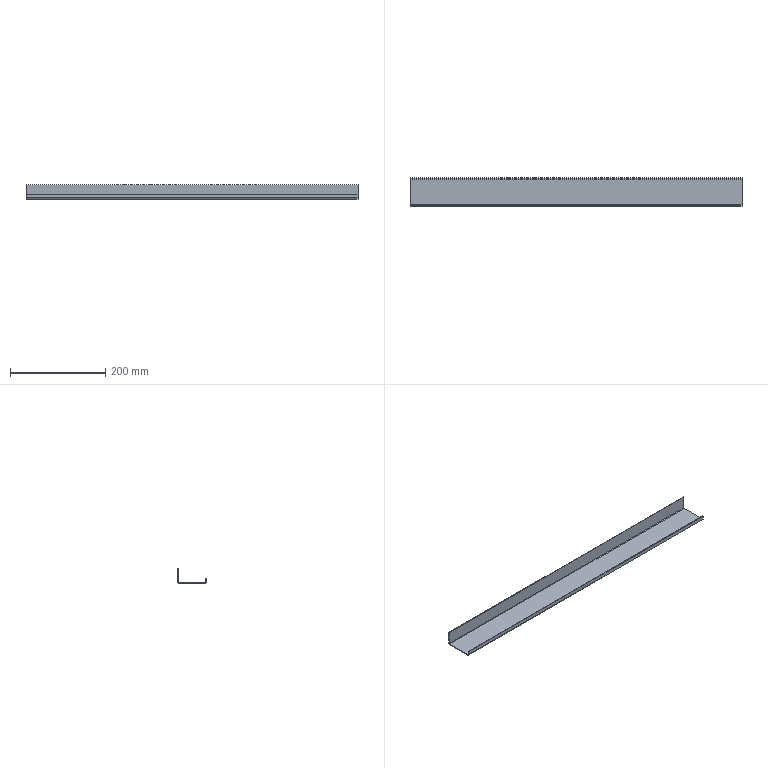Part | STEP file | 1 solid | 22 faces | box 697 x 59 x 30 mm | volume 98797 mm3 | plane 18 | cylinder 4 | commonest cylinder face diameters 2 x2 5 x2
STEP:
#1=CARTESIAN_POINT('',(0.,0.,0.));
#2=DIRECTION('',(0.,0.,1.));
#3=DIRECTION('',(1.,0.,0.));
#4=AXIS2_PLACEMENT_3D('',#1,#2,#3);
#5=CARTESIAN_POINT('',(697.,-56.5,-28.5));
#6=VERTEX_POINT('',#5);
#7=CARTESIAN_POINT('',(697.,-56.5,-30.));
#8=VERTEX_POINT('',#7);
#9=CARTESIAN_POINT('',(697.,-56.5,-28.5));
#10=DIRECTION('',(0.,0.,-1.));
#11=VECTOR('',#10,1.);
#12=LINE('',#9,#11);
#13=CARTESIAN_POINT('',(697.,-59.,-30.));
#14=DIRECTION('',(-1.,0.,0.));
#15=DIRECTION('',(0.,0.,1.));
#16=AXIS2_PLACEMENT_3D('',#13,#14,#15);
#17=PLANE('',#16);
#18=CARTESIAN_POINT('',(1.5,2.5));
#19=DIRECTION('',(-1.,0.));
#20=VECTOR('',#19,1.);
#21=LINE('',#18,#20);
#22=(GEOMETRIC_REPRESENTATION_CONTEXT(2)PARAMETRIC_REPRESENTATION_CONTEXT()REPRESENTATION_CONTEXT('',''));
#23=DEFINITIONAL_REPRESENTATION('',(#21),#22);
#24=PCURVE('',#17,#23);
#25=CARTESIAN_POINT('',(697.,-56.5,-27.5));
#26=DIRECTION('',(-1.,0.,0.));
#27=DIRECTION('',(0.,0.,1.));
#28=AXIS2_PLACEMENT_3D('',#25,#26,#27);
#29=PLANE('',#28);
#30=CARTESIAN_POINT('',(-1.,0.));
#31=DIRECTION('',(-1.,0.));
#32=VECTOR('',#31,1.);
#33=LINE('',#30,#32);
#34=(GEOMETRIC_REPRESENTATION_CONTEXT(2)PARAMETRIC_REPRESENTATION_CONTEXT()REPRESENTATION_CONTEXT('',''));
#35=DEFINITIONAL_REPRESENTATION('',(#33),#34);
#36=PCURVE('',#29,#35);
#37=SURFACE_CURVE('',#12,(#24,#36),.PCURVE_S1.);
#38=EDGE_CURVE('',#6,#8,#37,.T.);
#39=ORIENTED_EDGE('',*,*,#38,.T.);
#40=CARTESIAN_POINT('',(697.,-2.5,-30.));
#41=VERTEX_POINT('',#40);
#42=CARTESIAN_POINT('',(697.,0.,-30.));
#43=DIRECTION('',(0.,-1.,0.));
#44=VECTOR('',#43,1.);
#45=LINE('',#42,#44);
#46=CARTESIAN_POINT('',(0.,59.));
#47=DIRECTION('',(0.,-1.));
#48=VECTOR('',#47,1.);
#49=LINE('',#46,#48);
#50=(GEOMETRIC_REPRESENTATION_CONTEXT(2)PARAMETRIC_REPRESENTATION_CONTEXT()REPRESENTATION_CONTEXT('',''));
#51=DEFINITIONAL_REPRESENTATION('',(#49),#50);
#52=PCURVE('',#17,#51);
#53=CARTESIAN_POINT('',(0.,0.,-30.));
#54=DIRECTION('',(0.,0.,1.));
#55=DIRECTION('',(0.,-1.,0.));
#56=AXIS2_PLACEMENT_3D('',#53,#54,#55);
#57=PLANE('',#56);
#58=CARTESIAN_POINT('',(0.,697.));
#59=DIRECTION('',(1.,0.));
#60=VECTOR('',#59,1.);
#61=LINE('',#58,#60);
#62=(GEOMETRIC_REPRESENTATION_CONTEXT(2)PARAMETRIC_REPRESENTATION_CONTEXT()REPRESENTATION_CONTEXT('',''));
#63=DEFINITIONAL_REPRESENTATION('',(#61),#62);
#64=PCURVE('',#57,#63);
#65=SURFACE_CURVE('',#45,(#52,#64),.PCURVE_S1.);
#66=EDGE_CURVE('',#41,#8,#65,.T.);
#67=ORIENTED_EDGE('',*,*,#66,.F.);
#68=CARTESIAN_POINT('',(697.,-2.5,-28.5));
#69=VERTEX_POINT('',#68);
#70=CARTESIAN_POINT('',(697.,-2.5,-28.5));
#71=DIRECTION('',(0.,0.,-1.));
#72=VECTOR('',#71,1.);
#73=LINE('',#70,#72);
#74=CARTESIAN_POINT('',(1.5,56.5));
#75=DIRECTION('',(-1.,0.));
#76=VECTOR('',#75,1.);
#77=LINE('',#74,#76);
#78=(GEOMETRIC_REPRESENTATION_CONTEXT(2)PARAMETRIC_REPRESENTATION_CONTEXT()REPRESENTATION_CONTEXT('',''));
#79=DEFINITIONAL_REPRESENTATION('',(#77),#78);
#80=PCURVE('',#17,#79);
#81=CARTESIAN_POINT('',(697.,-2.5,-27.5));
#82=DIRECTION('',(-1.,0.,0.));
#83=DIRECTION('',(0.,0.,1.));
#84=AXIS2_PLACEMENT_3D('',#81,#82,#83);
#85=PLANE('',#84);
#86=CARTESIAN_POINT('',(-1.,0.));
#87=DIRECTION('',(-1.,0.));
#88=VECTOR('',#87,1.);
#89=LINE('',#86,#88);
#90=(GEOMETRIC_REPRESENTATION_CONTEXT(2)PARAMETRIC_REPRESENTATION_CONTEXT()REPRESENTATION_CONTEXT('',''));
#91=DEFINITIONAL_REPRESENTATION('',(#89),#90);
#92=PCURVE('',#85,#91);
#93=SURFACE_CURVE('',#73,(#80,#92),.PCURVE_S1.);
#94=EDGE_CURVE('',#69,#41,#93,.T.);
#95=ORIENTED_EDGE('',*,*,#94,.F.);
#96=CARTESIAN_POINT('',(697.,-59.,-28.5));
#97=DIRECTION('',(0.,-1.,0.));
#98=VECTOR('',#97,1.);
#99=LINE('',#96,#98);
#100=CARTESIAN_POINT('',(1.5,0.));
#101=DIRECTION('',(0.,-1.));
#102=VECTOR('',#101,1.);
#103=LINE('',#100,#102);
#104=(GEOMETRIC_REPRESENTATION_CONTEXT(2)PARAMETRIC_REPRESENTATION_CONTEXT()REPRESENTATION_CONTEXT('',''));
#105=DEFINITIONAL_REPRESENTATION('',(#103),#104);
#106=PCURVE('',#17,#105);
#107=CARTESIAN_POINT('',(0.,0.,-28.5));
#108=DIRECTION('',(0.,0.,1.));
#109=DIRECTION('',(0.,-1.,0.));
#110=AXIS2_PLACEMENT_3D('',#107,#108,#109);
#111=PLANE('',#110);
#112=CARTESIAN_POINT('',(59.,697.));
#113=DIRECTION('',(1.,0.));
#114=VECTOR('',#113,1.);
#115=LINE('',#112,#114);
#116=(GEOMETRIC_REPRESENTATION_CONTEXT(2)PARAMETRIC_REPRESENTATION_CONTEXT()REPRESENTATION_CONTEXT('',''));
#117=DEFINITIONAL_REPRESENTATION('',(#115),#116);
#118=PCURVE('',#111,#117);
#119=SURFACE_CURVE('',#99,(#106,#118),.PCURVE_S1.);
#120=EDGE_CURVE('',#69,#6,#119,.T.);
#121=ORIENTED_EDGE('',*,*,#120,.T.);
#122=EDGE_LOOP('',(#39,#67,#95,#121));
#123=FACE_BOUND('',#122,.T.);
#124=ADVANCED_FACE('',(#123),#17,.F.);
#125=CARTESIAN_POINT('',(0.,-56.5,-28.5));
#126=VERTEX_POINT('',#125);
#127=CARTESIAN_POINT('',(0.,-56.5,-30.));
#128=VERTEX_POINT('',#127);
#129=CARTESIAN_POINT('',(0.,-56.5,-28.5));
#130=DIRECTION('',(0.,0.,-1.));
#131=VECTOR('',#130,1.);
#132=LINE('',#129,#131);
#133=CARTESIAN_POINT('',(0.,-1.5,-30.));
#134=DIRECTION('',(1.,0.,0.));
#135=DIRECTION('',(0.,1.,0.));
#136=AXIS2_PLACEMENT_3D('',#133,#134,#135);
#137=PLANE('',#136);
#138=CARTESIAN_POINT('',(-55.,1.5));
#139=DIRECTION('',(0.,-1.));
#140=VECTOR('',#139,1.);
#141=LINE('',#138,#140);
#142=(GEOMETRIC_REPRESENTATION_CONTEXT(2)PARAMETRIC_REPRESENTATION_CONTEXT()REPRESENTATION_CONTEXT('',''));
#143=DEFINITIONAL_REPRESENTATION('',(#141),#142);
#144=PCURVE('',#137,#143);
#145=CARTESIAN_POINT('',(0.,-56.5,-27.5));
#146=DIRECTION('',(-1.,0.,0.));
#147=DIRECTION('',(0.,0.,1.));
#148=AXIS2_PLACEMENT_3D('',#145,#146,#147);
#149=PLANE('',#148);
#150=CARTESIAN_POINT('',(-1.,0.));
#151=DIRECTION('',(-1.,0.));
#152=VECTOR('',#151,1.);
#153=LINE('',#150,#152);
#154=(GEOMETRIC_REPRESENTATION_CONTEXT(2)PARAMETRIC_REPRESENTATION_CONTEXT()REPRESENTATION_CONTEXT('',''));
#155=DEFINITIONAL_REPRESENTATION('',(#153),#154);
#156=PCURVE('',#149,#155);
#157=SURFACE_CURVE('',#132,(#144,#156),.PCURVE_S1.);
#158=EDGE_CURVE('',#126,#128,#157,.T.);
#159=ORIENTED_EDGE('',*,*,#158,.F.);
#160=CARTESIAN_POINT('',(0.,-2.5,-28.5));
#161=VERTEX_POINT('',#160);
#162=CARTESIAN_POINT('',(0.,-1.5,-28.5));
#163=DIRECTION('',(0.,1.,0.));
#164=VECTOR('',#163,1.);
#165=LINE('',#162,#164);
#166=CARTESIAN_POINT('',(0.,1.5));
#167=DIRECTION('',(1.,0.));
#168=VECTOR('',#167,1.);
#169=LINE('',#166,#168);
#170=(GEOMETRIC_REPRESENTATION_CONTEXT(2)PARAMETRIC_REPRESENTATION_CONTEXT()REPRESENTATION_CONTEXT('',''));
#171=DEFINITIONAL_REPRESENTATION('',(#169),#170);
#172=PCURVE('',#137,#171);
#173=CARTESIAN_POINT('',(1.5,0.));
#174=DIRECTION('',(-1.,0.));
#175=VECTOR('',#174,1.);
#176=LINE('',#173,#175);
#177=(GEOMETRIC_REPRESENTATION_CONTEXT(2)PARAMETRIC_REPRESENTATION_CONTEXT()REPRESENTATION_CONTEXT('',''));
#178=DEFINITIONAL_REPRESENTATION('',(#176),#177);
#179=PCURVE('',#111,#178);
#180=SURFACE_CURVE('',#165,(#172,#179),.PCURVE_S1.);
#181=EDGE_CURVE('',#126,#161,#180,.T.);
#182=ORIENTED_EDGE('',*,*,#181,.T.);
#183=CARTESIAN_POINT('',(0.,-2.5,-30.));
#184=VERTEX_POINT('',#183);
#185=CARTESIAN_POINT('',(0.,-2.5,-30.));
#186=DIRECTION('',(0.,0.,-1.));
#187=VECTOR('',#186,1.);
#188=LINE('',#185,#187);
#189=CARTESIAN_POINT('',(-1.,0.));
#190=DIRECTION('',(0.,-1.));
#191=VECTOR('',#190,1.);
#192=LINE('',#189,#191);
#193=(GEOMETRIC_REPRESENTATION_CONTEXT(2)PARAMETRIC_REPRESENTATION_CONTEXT()REPRESENTATION_CONTEXT('',''));
#194=DEFINITIONAL_REPRESENTATION('',(#192),#193);
#195=PCURVE('',#137,#194);
#196=CARTESIAN_POINT('',(0.,-2.5,-27.5));
#197=DIRECTION('',(-1.,0.,0.));
#198=DIRECTION('',(0.,0.,1.));
#199=AXIS2_PLACEMENT_3D('',#196,#197,#198);
#200=PLANE('',#199);
#201=CARTESIAN_POINT('',(-2.5,0.));
#202=DIRECTION('',(-1.,0.));
#203=VECTOR('',#202,1.);
#204=LINE('',#201,#203);
#205=(GEOMETRIC_REPRESENTATION_CONTEXT(2)PARAMETRIC_REPRESENTATION_CONTEXT()REPRESENTATION_CONTEXT('',''));
#206=DEFINITIONAL_REPRESENTATION('',(#204),#205);
#207=PCURVE('',#200,#206);
#208=SURFACE_CURVE('',#188,(#195,#207),.PCURVE_S1.);
#209=EDGE_CURVE('',#161,#184,#208,.T.);
#210=ORIENTED_EDGE('',*,*,#209,.T.);
#211=CARTESIAN_POINT('',(0.,0.,-30.));
#212=DIRECTION('',(0.,1.,0.));
#213=VECTOR('',#212,1.);
#214=LINE('',#211,#213);
#215=CARTESIAN_POINT('',(1.5,0.));
#216=DIRECTION('',(1.,0.));
#217=VECTOR('',#216,1.);
#218=LINE('',#215,#217);
#219=(GEOMETRIC_REPRESENTATION_CONTEXT(2)PARAMETRIC_REPRESENTATION_CONTEXT()REPRESENTATION_CONTEXT('',''));
#220=DEFINITIONAL_REPRESENTATION('',(#218),#219);
#221=PCURVE('',#137,#220);
#222=CARTESIAN_POINT('',(0.,0.));
#223=DIRECTION('',(-1.,0.));
#224=VECTOR('',#223,1.);
#225=LINE('',#222,#224);
#226=(GEOMETRIC_REPRESENTATION_CONTEXT(2)PARAMETRIC_REPRESENTATION_CONTEXT()REPRESENTATION_CONTEXT('',''));
#227=DEFINITIONAL_REPRESENTATION('',(#225),#226);
#228=PCURVE('',#57,#227);
#229=SURFACE_CURVE('',#214,(#221,#228),.PCURVE_S1.);
#230=EDGE_CURVE('',#128,#184,#229,.T.);
#231=ORIENTED_EDGE('',*,*,#230,.F.);
#232=EDGE_LOOP('',(#159,#182,#210,#231));
#233=FACE_BOUND('',#232,.T.);
#234=ADVANCED_FACE('',(#233),#137,.F.);
#235=CARTESIAN_POINT('',(697.,-56.5,-30.));
#236=DIRECTION('',(-1.,0.,0.));
#237=VECTOR('',#236,1.);
#238=LINE('',#235,#237);
#239=CARTESIAN_POINT('',(56.5,697.));
#240=DIRECTION('',(0.,-1.));
#241=VECTOR('',#240,1.);
#242=LINE('',#239,#241);
#243=(GEOMETRIC_REPRESENTATION_CONTEXT(2)PARAMETRIC_REPRESENTATION_CONTEXT()REPRESENTATION_CONTEXT('',''));
#244=DEFINITIONAL_REPRESENTATION('',(#242),#243);
#245=PCURVE('',#57,#244);
#246=CARTESIAN_POINT('',(697.,-56.5,-27.5));
#247=DIRECTION('',(1.,0.,0.));
#248=DIRECTION('',(0.,-1.,0.));
#249=AXIS2_PLACEMENT_3D('',#246,#247,#248);
#250=CYLINDRICAL_SURFACE('',#249,2.5);
#251=CARTESIAN_POINT('',(1.571,0.));
#252=DIRECTION('',(0.,-1.));
#253=VECTOR('',#252,1.);
#254=LINE('',#251,#253);
#255=(GEOMETRIC_REPRESENTATION_CONTEXT(2)PARAMETRIC_REPRESENTATION_CONTEXT()REPRESENTATION_CONTEXT('',''));
#256=DEFINITIONAL_REPRESENTATION('',(#254),#255);
#257=PCURVE('',#250,#256);
#258=SURFACE_CURVE('',#238,(#245,#257),.PCURVE_S1.);
#259=EDGE_CURVE('',#8,#128,#258,.T.);
#260=ORIENTED_EDGE('',*,*,#259,.T.);
#261=ORIENTED_EDGE('',*,*,#230,.T.);
#262=CARTESIAN_POINT('',(0.,-2.5,-30.));
#263=DIRECTION('',(-1.,0.,0.));
#264=VECTOR('',#263,1.);
#265=LINE('',#262,#264);
#266=CARTESIAN_POINT('',(2.5,0.));
#267=DIRECTION('',(0.,-1.));
#268=VECTOR('',#267,1.);
#269=LINE('',#266,#268);
#270=(GEOMETRIC_REPRESENTATION_CONTEXT(2)PARAMETRIC_REPRESENTATION_CONTEXT()REPRESENTATION_CONTEXT('',''));
#271=DEFINITIONAL_REPRESENTATION('',(#269),#270);
#272=PCURVE('',#57,#271);
#273=CARTESIAN_POINT('',(697.,-2.5,-27.5));
#274=DIRECTION('',(1.,0.,0.));
#275=DIRECTION('',(0.,0.,-1.));
#276=AXIS2_PLACEMENT_3D('',#273,#274,#275);
#277=CYLINDRICAL_SURFACE('',#276,2.5);
#278=CARTESIAN_POINT('',(0.,-697.));
#279=DIRECTION('',(0.,-1.));
#280=VECTOR('',#279,1.);
#281=LINE('',#278,#280);
#282=(GEOMETRIC_REPRESENTATION_CONTEXT(2)PARAMETRIC_REPRESENTATION_CONTEXT()REPRESENTATION_CONTEXT('',''));
#283=DEFINITIONAL_REPRESENTATION('',(#281),#282);
#284=PCURVE('',#277,#283);
#285=SURFACE_CURVE('',#265,(#272,#284),.PCURVE_S1.);
#286=EDGE_CURVE('',#41,#184,#285,.T.);
#287=ORIENTED_EDGE('',*,*,#286,.F.);
#288=ORIENTED_EDGE('',*,*,#66,.T.);
#289=EDGE_LOOP('',(#260,#261,#287,#288));
#290=FACE_BOUND('',#289,.T.);
#291=ADVANCED_FACE('',(#290),#57,.F.);
#292=ORIENTED_EDGE('',*,*,#181,.F.);
#293=CARTESIAN_POINT('',(697.,-56.5,-28.5));
#294=DIRECTION('',(-1.,0.,0.));
#295=VECTOR('',#294,1.);
#296=LINE('',#293,#295);
#297=CARTESIAN_POINT('',(56.5,697.));
#298=DIRECTION('',(0.,-1.));
#299=VECTOR('',#298,1.);
#300=LINE('',#297,#299);
#301=(GEOMETRIC_REPRESENTATION_CONTEXT(2)PARAMETRIC_REPRESENTATION_CONTEXT()REPRESENTATION_CONTEXT('',''));
#302=DEFINITIONAL_REPRESENTATION('',(#300),#301);
#303=PCURVE('',#111,#302);
#304=CARTESIAN_POINT('',(697.,-56.5,-27.5));
#305=DIRECTION('',(1.,0.,0.));
#306=DIRECTION('',(0.,-1.,0.));
#307=AXIS2_PLACEMENT_3D('',#304,#305,#306);
#308=CYLINDRICAL_SURFACE('',#307,1.);
#309=CARTESIAN_POINT('',(1.571,0.));
#310=DIRECTION('',(0.,-1.));
#311=VECTOR('',#310,1.);
#312=LINE('',#309,#311);
#313=(GEOMETRIC_REPRESENTATION_CONTEXT(2)PARAMETRIC_REPRESENTATION_CONTEXT()REPRESENTATION_CONTEXT('',''));
#314=DEFINITIONAL_REPRESENTATION('',(#312),#313);
#315=PCURVE('',#308,#314);
#316=SURFACE_CURVE('',#296,(#303,#315),.PCURVE_S1.);
#317=EDGE_CURVE('',#6,#126,#316,.T.);
#318=ORIENTED_EDGE('',*,*,#317,.F.);
#319=ORIENTED_EDGE('',*,*,#120,.F.);
#320=CARTESIAN_POINT('',(0.,-2.5,-28.5));
#321=DIRECTION('',(1.,0.,0.));
#322=VECTOR('',#321,1.);
#323=LINE('',#320,#322);
#324=CARTESIAN_POINT('',(2.5,0.));
#325=DIRECTION('',(0.,1.));
#326=VECTOR('',#325,1.);
#327=LINE('',#324,#326);
#328=(GEOMETRIC_REPRESENTATION_CONTEXT(2)PARAMETRIC_REPRESENTATION_CONTEXT()REPRESENTATION_CONTEXT('',''));
#329=DEFINITIONAL_REPRESENTATION('',(#327),#328);
#330=PCURVE('',#111,#329);
#331=CARTESIAN_POINT('',(697.,-2.5,-27.5));
#332=DIRECTION('',(1.,0.,0.));
#333=DIRECTION('',(0.,0.,-1.));
#334=AXIS2_PLACEMENT_3D('',#331,#332,#333);
#335=CYLINDRICAL_SURFACE('',#334,1.);
#336=CARTESIAN_POINT('',(0.,-697.));
#337=DIRECTION('',(0.,1.));
#338=VECTOR('',#337,1.);
#339=LINE('',#336,#338);
#340=(GEOMETRIC_REPRESENTATION_CONTEXT(2)PARAMETRIC_REPRESENTATION_CONTEXT()REPRESENTATION_CONTEXT('',''));
#341=DEFINITIONAL_REPRESENTATION('',(#339),#340);
#342=PCURVE('',#335,#341);
#343=SURFACE_CURVE('',#323,(#330,#342),.PCURVE_S1.);
#344=EDGE_CURVE('',#161,#69,#343,.T.);
#345=ORIENTED_EDGE('',*,*,#344,.F.);
#346=EDGE_LOOP('',(#292,#318,#319,#345));
#347=FACE_BOUND('',#346,.T.);
#348=ADVANCED_FACE('',(#347),#111,.T.);
#349=CARTESIAN_POINT('',(697.,-1.5,0.));
#350=VERTEX_POINT('',#349);
#351=CARTESIAN_POINT('',(697.,-1.5,-27.5));
#352=VERTEX_POINT('',#351);
#353=CARTESIAN_POINT('',(697.,-1.5,-30.));
#354=DIRECTION('',(0.,0.,-1.));
#355=VECTOR('',#354,1.);
#356=LINE('',#353,#355);
#357=CARTESIAN_POINT('',(697.,-1.5,-30.));
#358=DIRECTION('',(1.,0.,0.));
#359=DIRECTION('',(0.,0.,-1.));
#360=AXIS2_PLACEMENT_3D('',#357,#358,#359);
#361=PLANE('',#360);
#362=CARTESIAN_POINT('',(0.,0.));
#363=DIRECTION('',(1.,0.));
#364=VECTOR('',#363,1.);
#365=LINE('',#362,#364);
#366=(GEOMETRIC_REPRESENTATION_CONTEXT(2)PARAMETRIC_REPRESENTATION_CONTEXT()REPRESENTATION_CONTEXT('',''));
#367=DEFINITIONAL_REPRESENTATION('',(#365),#366);
#368=PCURVE('',#361,#367);
#369=CARTESIAN_POINT('',(0.,-1.5,0.));
#370=DIRECTION('',(0.,1.,0.));
#371=DIRECTION('',(0.,0.,1.));
#372=AXIS2_PLACEMENT_3D('',#369,#370,#371);
#373=PLANE('',#372);
#374=CARTESIAN_POINT('',(-30.,697.));
#375=DIRECTION('',(-1.,0.));
#376=VECTOR('',#375,1.);
#377=LINE('',#374,#376);
#378=(GEOMETRIC_REPRESENTATION_CONTEXT(2)PARAMETRIC_REPRESENTATION_CONTEXT()REPRESENTATION_CONTEXT('',''));
#379=DEFINITIONAL_REPRESENTATION('',(#377),#378);
#380=PCURVE('',#373,#379);
#381=SURFACE_CURVE('',#356,(#368,#380),.PCURVE_S1.);
#382=EDGE_CURVE('',#350,#352,#381,.T.);
#383=ORIENTED_EDGE('',*,*,#382,.T.);
#384=CARTESIAN_POINT('',(697.,0.,-27.5));
#385=VERTEX_POINT('',#384);
#386=CARTESIAN_POINT('',(697.,-1.5,-27.5));
#387=DIRECTION('',(0.,1.,0.));
#388=VECTOR('',#387,1.);
#389=LINE('',#386,#388);
#390=CARTESIAN_POINT('',(-2.5,0.));
#391=DIRECTION('',(0.,1.));
#392=VECTOR('',#391,1.);
#393=LINE('',#390,#392);
#394=(GEOMETRIC_REPRESENTATION_CONTEXT(2)PARAMETRIC_REPRESENTATION_CONTEXT()REPRESENTATION_CONTEXT('',''));
#395=DEFINITIONAL_REPRESENTATION('',(#393),#394);
#396=PCURVE('',#361,#395);
#397=CARTESIAN_POINT('',(0.,1.));
#398=DIRECTION('',(0.,1.));
#399=VECTOR('',#398,1.);
#400=LINE('',#397,#399);
#401=(GEOMETRIC_REPRESENTATION_CONTEXT(2)PARAMETRIC_REPRESENTATION_CONTEXT()REPRESENTATION_CONTEXT('',''));
#402=DEFINITIONAL_REPRESENTATION('',(#400),#401);
#403=PCURVE('',#85,#402);
#404=SURFACE_CURVE('',#389,(#396,#403),.PCURVE_S1.);
#405=EDGE_CURVE('',#352,#385,#404,.T.);
#406=ORIENTED_EDGE('',*,*,#405,.T.);
#407=CARTESIAN_POINT('',(697.,0.,0.));
#408=VERTEX_POINT('',#407);
#409=CARTESIAN_POINT('',(697.,0.,-30.));
#410=DIRECTION('',(0.,0.,-1.));
#411=VECTOR('',#410,1.);
#412=LINE('',#409,#411);
#413=CARTESIAN_POINT('',(0.,1.5));
#414=DIRECTION('',(1.,0.));
#415=VECTOR('',#414,1.);
#416=LINE('',#413,#415);
#417=(GEOMETRIC_REPRESENTATION_CONTEXT(2)PARAMETRIC_REPRESENTATION_CONTEXT()REPRESENTATION_CONTEXT('',''));
#418=DEFINITIONAL_REPRESENTATION('',(#416),#417);
#419=PCURVE('',#361,#418);
#420=CARTESIAN_POINT('',(0.,0.,0.));
#421=DIRECTION('',(0.,1.,0.));
#422=DIRECTION('',(0.,0.,1.));
#423=AXIS2_PLACEMENT_3D('',#420,#421,#422);
#424=PLANE('',#423);
#425=CARTESIAN_POINT('',(-30.,697.));
#426=DIRECTION('',(-1.,0.));
#427=VECTOR('',#426,1.);
#428=LINE('',#425,#427);
#429=(GEOMETRIC_REPRESENTATION_CONTEXT(2)PARAMETRIC_REPRESENTATION_CONTEXT()REPRESENTATION_CONTEXT('',''));
#430=DEFINITIONAL_REPRESENTATION('',(#428),#429);
#431=PCURVE('',#424,#430);
#432=SURFACE_CURVE('',#412,(#419,#431),.PCURVE_S1.);
#433=EDGE_CURVE('',#408,#385,#432,.T.);
#434=ORIENTED_EDGE('',*,*,#433,.F.);
#435=CARTESIAN_POINT('',(697.,-1.5,0.));
#436=DIRECTION('',(0.,1.,0.));
#437=VECTOR('',#436,1.);
#438=LINE('',#435,#437);
#439=CARTESIAN_POINT('',(-30.,0.));
#440=DIRECTION('',(0.,1.));
#441=VECTOR('',#440,1.);
#442=LINE('',#439,#441);
#443=(GEOMETRIC_REPRESENTATION_CONTEXT(2)PARAMETRIC_REPRESENTATION_CONTEXT()REPRESENTATION_CONTEXT('',''));
#444=DEFINITIONAL_REPRESENTATION('',(#442),#443);
#445=PCURVE('',#361,#444);
#446=CARTESIAN_POINT('',(0.,-1.5,0.));
#447=DIRECTION('',(0.,0.,1.));
#448=DIRECTION('',(1.,0.,0.));
#449=AXIS2_PLACEMENT_3D('',#446,#447,#448);
#450=PLANE('',#449);
#451=CARTESIAN_POINT('',(697.,0.));
#452=DIRECTION('',(0.,1.));
#453=VECTOR('',#452,1.);
#454=LINE('',#451,#453);
#455=(GEOMETRIC_REPRESENTATION_CONTEXT(2)PARAMETRIC_REPRESENTATION_CONTEXT()REPRESENTATION_CONTEXT('',''));
#456=DEFINITIONAL_REPRESENTATION('',(#454),#455);
#457=PCURVE('',#450,#456);
#458=SURFACE_CURVE('',#438,(#445,#457),.PCURVE_S1.);
#459=EDGE_CURVE('',#350,#408,#458,.T.);
#460=ORIENTED_EDGE('',*,*,#459,.F.);
#461=EDGE_LOOP('',(#383,#406,#434,#460));
#462=FACE_BOUND('',#461,.T.);
#463=ADVANCED_FACE('',(#462),#361,.T.);
#464=CARTESIAN_POINT('',(0.,-1.5,-27.5));
#465=VERTEX_POINT('',#464);
#466=CARTESIAN_POINT('',(697.,-1.5,-27.5));
#467=DIRECTION('',(-1.,0.,0.));
#468=VECTOR('',#467,1.);
#469=LINE('',#466,#468);
#470=CARTESIAN_POINT('',(-27.5,697.));
#471=DIRECTION('',(0.,-1.));
#472=VECTOR('',#471,1.);
#473=LINE('',#470,#472);
#474=(GEOMETRIC_REPRESENTATION_CONTEXT(2)PARAMETRIC_REPRESENTATION_CONTEXT()REPRESENTATION_CONTEXT('',''));
#475=DEFINITIONAL_REPRESENTATION('',(#473),#474);
#476=PCURVE('',#373,#475);
#477=CARTESIAN_POINT('',(1.571,0.));
#478=DIRECTION('',(0.,-1.));
#479=VECTOR('',#478,1.);
#480=LINE('',#477,#479);
#481=(GEOMETRIC_REPRESENTATION_CONTEXT(2)PARAMETRIC_REPRESENTATION_CONTEXT()REPRESENTATION_CONTEXT('',''));
#482=DEFINITIONAL_REPRESENTATION('',(#480),#481);
#483=PCURVE('',#335,#482);
#484=SURFACE_CURVE('',#469,(#476,#483),.PCURVE_S1.);
#485=EDGE_CURVE('',#352,#465,#484,.T.);
#486=ORIENTED_EDGE('',*,*,#485,.F.);
#487=ORIENTED_EDGE('',*,*,#382,.F.);
#488=CARTESIAN_POINT('',(0.,-1.5,0.));
#489=VERTEX_POINT('',#488);
#490=CARTESIAN_POINT('',(0.,-1.5,0.));
#491=DIRECTION('',(1.,0.,0.));
#492=VECTOR('',#491,1.);
#493=LINE('',#490,#492);
#494=CARTESIAN_POINT('',(0.,0.));
#495=DIRECTION('',(0.,1.));
#496=VECTOR('',#495,1.);
#497=LINE('',#494,#496);
#498=(GEOMETRIC_REPRESENTATION_CONTEXT(2)PARAMETRIC_REPRESENTATION_CONTEXT()REPRESENTATION_CONTEXT('',''));
#499=DEFINITIONAL_REPRESENTATION('',(#497),#498);
#500=PCURVE('',#373,#499);
#501=CARTESIAN_POINT('',(0.,0.));
#502=DIRECTION('',(1.,0.));
#503=VECTOR('',#502,1.);
#504=LINE('',#501,#503);
#505=(GEOMETRIC_REPRESENTATION_CONTEXT(2)PARAMETRIC_REPRESENTATION_CONTEXT()REPRESENTATION_CONTEXT('',''));
#506=DEFINITIONAL_REPRESENTATION('',(#504),#505);
#507=PCURVE('',#450,#506);
#508=SURFACE_CURVE('',#493,(#500,#507),.PCURVE_S1.);
#509=EDGE_CURVE('',#489,#350,#508,.T.);
#510=ORIENTED_EDGE('',*,*,#509,.F.);
#511=CARTESIAN_POINT('',(0.,-1.5,-30.));
#512=DIRECTION('',(0.,0.,1.));
#513=VECTOR('',#512,1.);
#514=LINE('',#511,#513);
#515=CARTESIAN_POINT('',(-30.,0.));
#516=DIRECTION('',(1.,0.));
#517=VECTOR('',#516,1.);
#518=LINE('',#515,#517);
#519=(GEOMETRIC_REPRESENTATION_CONTEXT(2)PARAMETRIC_REPRESENTATION_CONTEXT()REPRESENTATION_CONTEXT('',''));
#520=DEFINITIONAL_REPRESENTATION('',(#518),#519);
#521=PCURVE('',#373,#520);
#522=CARTESIAN_POINT('',(0.,-1.5,-30.));
#523=DIRECTION('',(-1.,0.,0.));
#524=DIRECTION('',(0.,0.,1.));
#525=AXIS2_PLACEMENT_3D('',#522,#523,#524);
#526=PLANE('',#525);
#527=CARTESIAN_POINT('',(0.,0.));
#528=DIRECTION('',(1.,0.));
#529=VECTOR('',#528,1.);
#530=LINE('',#527,#529);
#531=(GEOMETRIC_REPRESENTATION_CONTEXT(2)PARAMETRIC_REPRESENTATION_CONTEXT()REPRESENTATION_CONTEXT('',''));
#532=DEFINITIONAL_REPRESENTATION('',(#530),#531);
#533=PCURVE('',#526,#532);
#534=SURFACE_CURVE('',#514,(#521,#533),.PCURVE_S1.);
#535=EDGE_CURVE('',#465,#489,#534,.T.);
#536=ORIENTED_EDGE('',*,*,#535,.F.);
#537=EDGE_LOOP('',(#486,#487,#510,#536));
#538=FACE_BOUND('',#537,.T.);
#539=ADVANCED_FACE('',(#538),#373,.F.);
#540=ORIENTED_EDGE('',*,*,#433,.T.);
#541=CARTESIAN_POINT('',(0.,0.,-27.5));
#542=VERTEX_POINT('',#541);
#543=CARTESIAN_POINT('',(697.,0.,-27.5));
#544=DIRECTION('',(-1.,0.,0.));
#545=VECTOR('',#544,1.);
#546=LINE('',#543,#545);
#547=CARTESIAN_POINT('',(-27.5,697.));
#548=DIRECTION('',(0.,-1.));
#549=VECTOR('',#548,1.);
#550=LINE('',#547,#549);
#551=(GEOMETRIC_REPRESENTATION_CONTEXT(2)PARAMETRIC_REPRESENTATION_CONTEXT()REPRESENTATION_CONTEXT('',''));
#552=DEFINITIONAL_REPRESENTATION('',(#550),#551);
#553=PCURVE('',#424,#552);
#554=CARTESIAN_POINT('',(1.571,0.));
#555=DIRECTION('',(0.,-1.));
#556=VECTOR('',#555,1.);
#557=LINE('',#554,#556);
#558=(GEOMETRIC_REPRESENTATION_CONTEXT(2)PARAMETRIC_REPRESENTATION_CONTEXT()REPRESENTATION_CONTEXT('',''));
#559=DEFINITIONAL_REPRESENTATION('',(#557),#558);
#560=PCURVE('',#277,#559);
#561=SURFACE_CURVE('',#546,(#553,#560),.PCURVE_S1.);
#562=EDGE_CURVE('',#385,#542,#561,.T.);
#563=ORIENTED_EDGE('',*,*,#562,.T.);
#564=CARTESIAN_POINT('',(0.,0.,0.));
#565=VERTEX_POINT('',#564);
#566=CARTESIAN_POINT('',(0.,0.,-30.));
#567=DIRECTION('',(0.,0.,1.));
#568=VECTOR('',#567,1.);
#569=LINE('',#566,#568);
#570=CARTESIAN_POINT('',(-30.,0.));
#571=DIRECTION('',(1.,0.));
#572=VECTOR('',#571,1.);
#573=LINE('',#570,#572);
#574=(GEOMETRIC_REPRESENTATION_CONTEXT(2)PARAMETRIC_REPRESENTATION_CONTEXT()REPRESENTATION_CONTEXT('',''));
#575=DEFINITIONAL_REPRESENTATION('',(#573),#574);
#576=PCURVE('',#424,#575);
#577=CARTESIAN_POINT('',(0.,1.5));
#578=DIRECTION('',(1.,0.));
#579=VECTOR('',#578,1.);
#580=LINE('',#577,#579);
#581=(GEOMETRIC_REPRESENTATION_CONTEXT(2)PARAMETRIC_REPRESENTATION_CONTEXT()REPRESENTATION_CONTEXT('',''));
#582=DEFINITIONAL_REPRESENTATION('',(#580),#581);
#583=PCURVE('',#526,#582);
#584=SURFACE_CURVE('',#569,(#576,#583),.PCURVE_S1.);
#585=EDGE_CURVE('',#542,#565,#584,.T.);
#586=ORIENTED_EDGE('',*,*,#585,.T.);
#587=CARTESIAN_POINT('',(0.,0.,0.));
#588=DIRECTION('',(1.,0.,0.));
#589=VECTOR('',#588,1.);
#590=LINE('',#587,#589);
#591=CARTESIAN_POINT('',(0.,0.));
#592=DIRECTION('',(0.,1.));
#593=VECTOR('',#592,1.);
#594=LINE('',#591,#593);
#595=(GEOMETRIC_REPRESENTATION_CONTEXT(2)PARAMETRIC_REPRESENTATION_CONTEXT()REPRESENTATION_CONTEXT('',''));
#596=DEFINITIONAL_REPRESENTATION('',(#594),#595);
#597=PCURVE('',#424,#596);
#598=CARTESIAN_POINT('',(0.,1.5));
#599=DIRECTION('',(1.,0.));
#600=VECTOR('',#599,1.);
#601=LINE('',#598,#600);
#602=(GEOMETRIC_REPRESENTATION_CONTEXT(2)PARAMETRIC_REPRESENTATION_CONTEXT()REPRESENTATION_CONTEXT('',''));
#603=DEFINITIONAL_REPRESENTATION('',(#601),#602);
#604=PCURVE('',#450,#603);
#605=SURFACE_CURVE('',#590,(#597,#604),.PCURVE_S1.);
#606=EDGE_CURVE('',#565,#408,#605,.T.);
#607=ORIENTED_EDGE('',*,*,#606,.T.);
#608=EDGE_LOOP('',(#540,#563,#586,#607));
#609=FACE_BOUND('',#608,.T.);
#610=ADVANCED_FACE('',(#609),#424,.T.);
#611=CARTESIAN_POINT('',(0.,-1.5,-27.5));
#612=DIRECTION('',(0.,1.,0.));
#613=VECTOR('',#612,1.);
#614=LINE('',#611,#613);
#615=CARTESIAN_POINT('',(2.5,0.));
#616=DIRECTION('',(0.,1.));
#617=VECTOR('',#616,1.);
#618=LINE('',#615,#617);
#619=(GEOMETRIC_REPRESENTATION_CONTEXT(2)PARAMETRIC_REPRESENTATION_CONTEXT()REPRESENTATION_CONTEXT('',''));
#620=DEFINITIONAL_REPRESENTATION('',(#618),#619);
#621=PCURVE('',#526,#620);
#622=CARTESIAN_POINT('',(0.,1.));
#623=DIRECTION('',(0.,1.));
#624=VECTOR('',#623,1.);
#625=LINE('',#622,#624);
#626=(GEOMETRIC_REPRESENTATION_CONTEXT(2)PARAMETRIC_REPRESENTATION_CONTEXT()REPRESENTATION_CONTEXT('',''));
#627=DEFINITIONAL_REPRESENTATION('',(#625),#626);
#628=PCURVE('',#200,#627);
#629=SURFACE_CURVE('',#614,(#621,#628),.PCURVE_S1.);
#630=EDGE_CURVE('',#465,#542,#629,.T.);
#631=ORIENTED_EDGE('',*,*,#630,.F.);
#632=ORIENTED_EDGE('',*,*,#535,.T.);
#633=CARTESIAN_POINT('',(0.,-1.5,0.));
#634=DIRECTION('',(0.,1.,0.));
#635=VECTOR('',#634,1.);
#636=LINE('',#633,#635);
#637=CARTESIAN_POINT('',(30.,0.));
#638=DIRECTION('',(0.,1.));
#639=VECTOR('',#638,1.);
#640=LINE('',#637,#639);
#641=(GEOMETRIC_REPRESENTATION_CONTEXT(2)PARAMETRIC_REPRESENTATION_CONTEXT()REPRESENTATION_CONTEXT('',''));
#642=DEFINITIONAL_REPRESENTATION('',(#640),#641);
#643=PCURVE('',#526,#642);
#644=CARTESIAN_POINT('',(0.,0.));
#645=DIRECTION('',(0.,1.));
#646=VECTOR('',#645,1.);
#647=LINE('',#644,#646);
#648=(GEOMETRIC_REPRESENTATION_CONTEXT(2)PARAMETRIC_REPRESENTATION_CONTEXT()REPRESENTATION_CONTEXT('',''));
#649=DEFINITIONAL_REPRESENTATION('',(#647),#648);
#650=PCURVE('',#450,#649);
#651=SURFACE_CURVE('',#636,(#643,#650),.PCURVE_S1.);
#652=EDGE_CURVE('',#489,#565,#651,.T.);
#653=ORIENTED_EDGE('',*,*,#652,.T.);
#654=ORIENTED_EDGE('',*,*,#585,.F.);
#655=EDGE_LOOP('',(#631,#632,#653,#654));
#656=FACE_BOUND('',#655,.T.);
#657=ADVANCED_FACE('',(#656),#526,.T.);
#658=ORIENTED_EDGE('',*,*,#606,.F.);
#659=ORIENTED_EDGE('',*,*,#652,.F.);
#660=ORIENTED_EDGE('',*,*,#509,.T.);
#661=ORIENTED_EDGE('',*,*,#459,.T.);
#662=EDGE_LOOP('',(#658,#659,#660,#661));
#663=FACE_BOUND('',#662,.T.);
#664=ADVANCED_FACE('',(#663),#450,.T.);
#665=ORIENTED_EDGE('',*,*,#209,.F.);
#666=CARTESIAN_POINT('',(0.,-2.5,-27.5));
#667=DIRECTION('',(-1.,0.,0.));
#668=DIRECTION('',(0.,0.,-1.));
#669=AXIS2_PLACEMENT_3D('',#666,#667,#668);
#670=CIRCLE('',#669,1.);
#671=CARTESIAN_POINT('',(0.,0.));
#672=DIRECTION('',(-1.,0.));
#673=AXIS2_PLACEMENT_2D('',#671,#672);
#674=CIRCLE('',#673,1.);
#675=(GEOMETRIC_REPRESENTATION_CONTEXT(2)PARAMETRIC_REPRESENTATION_CONTEXT()REPRESENTATION_CONTEXT('',''));
#676=DEFINITIONAL_REPRESENTATION('',(#674),#675);
#677=PCURVE('',#200,#676);
#678=CARTESIAN_POINT('',(6.283,-697.));
#679=DIRECTION('',(-1.,0.));
#680=VECTOR('',#679,1.);
#681=LINE('',#678,#680);
#682=(GEOMETRIC_REPRESENTATION_CONTEXT(2)PARAMETRIC_REPRESENTATION_CONTEXT()REPRESENTATION_CONTEXT('',''));
#683=DEFINITIONAL_REPRESENTATION('',(#681),#682);
#684=PCURVE('',#335,#683);
#685=SURFACE_CURVE('',#670,(#677,#684),.PCURVE_S1.);
#686=EDGE_CURVE('',#465,#161,#685,.T.);
#687=ORIENTED_EDGE('',*,*,#686,.F.);
#688=ORIENTED_EDGE('',*,*,#630,.T.);
#689=CARTESIAN_POINT('',(0.,-2.5,-27.5));
#690=DIRECTION('',(-1.,0.,0.));
#691=DIRECTION('',(0.,0.,-1.));
#692=AXIS2_PLACEMENT_3D('',#689,#690,#691);
#693=CIRCLE('',#692,2.5);
#694=CARTESIAN_POINT('',(0.,0.));
#695=DIRECTION('',(-1.,0.));
#696=AXIS2_PLACEMENT_2D('',#694,#695);
#697=CIRCLE('',#696,2.5);
#698=(GEOMETRIC_REPRESENTATION_CONTEXT(2)PARAMETRIC_REPRESENTATION_CONTEXT()REPRESENTATION_CONTEXT('',''));
#699=DEFINITIONAL_REPRESENTATION('',(#697),#698);
#700=PCURVE('',#200,#699);
#701=CARTESIAN_POINT('',(6.283,-697.));
#702=DIRECTION('',(-1.,0.));
#703=VECTOR('',#702,1.);
#704=LINE('',#701,#703);
#705=(GEOMETRIC_REPRESENTATION_CONTEXT(2)PARAMETRIC_REPRESENTATION_CONTEXT()REPRESENTATION_CONTEXT('',''));
#706=DEFINITIONAL_REPRESENTATION('',(#704),#705);
#707=PCURVE('',#277,#706);
#708=SURFACE_CURVE('',#693,(#700,#707),.PCURVE_S1.);
#709=EDGE_CURVE('',#542,#184,#708,.T.);
#710=ORIENTED_EDGE('',*,*,#709,.T.);
#711=EDGE_LOOP('',(#665,#687,#688,#710));
#712=FACE_BOUND('',#711,.T.);
#713=ADVANCED_FACE('',(#712),#200,.T.);
#714=CARTESIAN_POINT('',(697.,-2.5,-27.5));
#715=DIRECTION('',(1.,0.,0.));
#716=DIRECTION('',(0.,0.,-1.));
#717=AXIS2_PLACEMENT_3D('',#714,#715,#716);
#718=CIRCLE('',#717,1.);
#719=CARTESIAN_POINT('',(-1.,0.));
#720=CARTESIAN_POINT('',(-1.,1.732));
#721=CARTESIAN_POINT('',(0.5,0.866));
#722=CARTESIAN_POINT('',(2.,0.));
#723=CARTESIAN_POINT('',(0.5,-0.866));
#724=CARTESIAN_POINT('',(-1.,-1.732));
#725=CARTESIAN_POINT('',(-1.,0.));
#726=(BOUNDED_CURVE()B_SPLINE_CURVE(2,(#719,#720,#721,#722,#723,#724,#725),.UNSPECIFIED.,.T.,.F.)B_SPLINE_CURVE_WITH_KNOTS((1,2,2,2,2,1),(-2.094,0.,2.094,4.189,6.283,8.378),.UNSPECIFIED.)CURVE()GEOMETRIC_REPRESENTATION_ITEM()RATIONAL_B_SPLINE_CURVE((1.,0.5,1.,0.5,1.,0.5,1.))REPRESENTATION_ITEM(''));
#727=(GEOMETRIC_REPRESENTATION_CONTEXT(2)PARAMETRIC_REPRESENTATION_CONTEXT()REPRESENTATION_CONTEXT('',''));
#728=DEFINITIONAL_REPRESENTATION('',(#726),#727);
#729=PCURVE('',#85,#728);
#730=CARTESIAN_POINT('',(0.,0.));
#731=DIRECTION('',(1.,0.));
#732=VECTOR('',#731,1.);
#733=LINE('',#730,#732);
#734=(GEOMETRIC_REPRESENTATION_CONTEXT(2)PARAMETRIC_REPRESENTATION_CONTEXT()REPRESENTATION_CONTEXT('',''));
#735=DEFINITIONAL_REPRESENTATION('',(#733),#734);
#736=PCURVE('',#335,#735);
#737=SURFACE_CURVE('',#718,(#729,#736),.PCURVE_S1.);
#738=EDGE_CURVE('',#69,#352,#737,.T.);
#739=ORIENTED_EDGE('',*,*,#738,.F.);
#740=ORIENTED_EDGE('',*,*,#94,.T.);
#741=CARTESIAN_POINT('',(697.,-2.5,-27.5));
#742=DIRECTION('',(1.,0.,0.));
#743=DIRECTION('',(0.,0.,-1.));
#744=AXIS2_PLACEMENT_3D('',#741,#742,#743);
#745=CIRCLE('',#744,2.5);
#746=CARTESIAN_POINT('',(-2.5,0.));
#747=CARTESIAN_POINT('',(-2.5,4.33));
#748=CARTESIAN_POINT('',(1.25,2.165));
#749=CARTESIAN_POINT('',(5.,0.));
#750=CARTESIAN_POINT('',(1.25,-2.165));
#751=CARTESIAN_POINT('',(-2.5,-4.33));
#752=CARTESIAN_POINT('',(-2.5,0.));
#753=(BOUNDED_CURVE()B_SPLINE_CURVE(2,(#746,#747,#748,#749,#750,#751,#752),.UNSPECIFIED.,.T.,.F.)B_SPLINE_CURVE_WITH_KNOTS((1,2,2,2,2,1),(-2.094,0.,2.094,4.189,6.283,8.378),.UNSPECIFIED.)CURVE()GEOMETRIC_REPRESENTATION_ITEM()RATIONAL_B_SPLINE_CURVE((1.,0.5,1.,0.5,1.,0.5,1.))REPRESENTATION_ITEM(''));
#754=(GEOMETRIC_REPRESENTATION_CONTEXT(2)PARAMETRIC_REPRESENTATION_CONTEXT()REPRESENTATION_CONTEXT('',''));
#755=DEFINITIONAL_REPRESENTATION('',(#753),#754);
#756=PCURVE('',#85,#755);
#757=CARTESIAN_POINT('',(0.,0.));
#758=DIRECTION('',(1.,0.));
#759=VECTOR('',#758,1.);
#760=LINE('',#757,#759);
#761=(GEOMETRIC_REPRESENTATION_CONTEXT(2)PARAMETRIC_REPRESENTATION_CONTEXT()REPRESENTATION_CONTEXT('',''));
#762=DEFINITIONAL_REPRESENTATION('',(#760),#761);
#763=PCURVE('',#277,#762);
#764=SURFACE_CURVE('',#745,(#756,#763),.PCURVE_S1.);
#765=EDGE_CURVE('',#41,#385,#764,.T.);
#766=ORIENTED_EDGE('',*,*,#765,.T.);
#767=ORIENTED_EDGE('',*,*,#405,.F.);
#768=EDGE_LOOP('',(#739,#740,#766,#767));
#769=FACE_BOUND('',#768,.T.);
#770=ADVANCED_FACE('',(#769),#85,.F.);
#771=ORIENTED_EDGE('',*,*,#562,.F.);
#772=ORIENTED_EDGE('',*,*,#765,.F.);
#773=ORIENTED_EDGE('',*,*,#286,.T.);
#774=ORIENTED_EDGE('',*,*,#709,.F.);
#775=EDGE_LOOP('',(#771,#772,#773,#774));
#776=FACE_BOUND('',#775,.T.);
#777=ADVANCED_FACE('',(#776),#277,.T.);
#778=ORIENTED_EDGE('',*,*,#738,.F.);
#779=ORIENTED_EDGE('',*,*,#344,.F.);
#780=ORIENTED_EDGE('',*,*,#686,.F.);
#781=ORIENTED_EDGE('',*,*,#485,.F.);
#782=EDGE_LOOP('',(#778,#779,#780,#781));
#783=FACE_BOUND('',#782,.F.);
#784=ADVANCED_FACE('',(#783),#335,.F.);
#785=CARTESIAN_POINT('',(0.,-57.5,-27.5));
#786=VERTEX_POINT('',#785);
#787=CARTESIAN_POINT('',(0.,-59.,-27.5));
#788=VERTEX_POINT('',#787);
#789=CARTESIAN_POINT('',(0.,-59.,-27.5));
#790=DIRECTION('',(0.,-1.,0.));
#791=VECTOR('',#790,1.);
#792=LINE('',#789,#791);
#793=CARTESIAN_POINT('',(0.,-2.5));
#794=DIRECTION('',(0.,-1.));
#795=VECTOR('',#794,1.);
#796=LINE('',#793,#795);
#797=(GEOMETRIC_REPRESENTATION_CONTEXT(2)PARAMETRIC_REPRESENTATION_CONTEXT()REPRESENTATION_CONTEXT('',''));
#798=DEFINITIONAL_REPRESENTATION('',(#796),#797);
#799=PCURVE('',#149,#798);
#800=CARTESIAN_POINT('',(0.,-59.,-28.5));
#801=DIRECTION('',(1.,0.,0.));
#802=DIRECTION('',(0.,0.,-1.));
#803=AXIS2_PLACEMENT_3D('',#800,#801,#802);
#804=PLANE('',#803);
#805=CARTESIAN_POINT('',(-1.,0.));
#806=DIRECTION('',(0.,-1.));
#807=VECTOR('',#806,1.);
#808=LINE('',#805,#807);
#809=(GEOMETRIC_REPRESENTATION_CONTEXT(2)PARAMETRIC_REPRESENTATION_CONTEXT()REPRESENTATION_CONTEXT('',''));
#810=DEFINITIONAL_REPRESENTATION('',(#808),#809);
#811=PCURVE('',#804,#810);
#812=SURFACE_CURVE('',#792,(#799,#811),.PCURVE_S1.);
#813=EDGE_CURVE('',#786,#788,#812,.T.);
#814=ORIENTED_EDGE('',*,*,#813,.F.);
#815=CARTESIAN_POINT('',(0.,-56.5,-27.5));
#816=DIRECTION('',(-1.,0.,0.));
#817=DIRECTION('',(0.,0.,-1.));
#818=AXIS2_PLACEMENT_3D('',#815,#816,#817);
#819=CIRCLE('',#818,1.);
#820=CARTESIAN_POINT('',(0.,0.));
#821=DIRECTION('',(-1.,0.));
#822=AXIS2_PLACEMENT_2D('',#820,#821);
#823=CIRCLE('',#822,1.);
#824=(GEOMETRIC_REPRESENTATION_CONTEXT(2)PARAMETRIC_REPRESENTATION_CONTEXT()REPRESENTATION_CONTEXT('',''));
#825=DEFINITIONAL_REPRESENTATION('',(#823),#824);
#826=PCURVE('',#149,#825);
#827=CARTESIAN_POINT('',(1.571,-697.));
#828=DIRECTION('',(-1.,0.));
#829=VECTOR('',#828,1.);
#830=LINE('',#827,#829);
#831=(GEOMETRIC_REPRESENTATION_CONTEXT(2)PARAMETRIC_REPRESENTATION_CONTEXT()REPRESENTATION_CONTEXT('',''));
#832=DEFINITIONAL_REPRESENTATION('',(#830),#831);
#833=PCURVE('',#308,#832);
#834=SURFACE_CURVE('',#819,(#826,#833),.PCURVE_S1.);
#835=EDGE_CURVE('',#126,#786,#834,.T.);
#836=ORIENTED_EDGE('',*,*,#835,.F.);
#837=ORIENTED_EDGE('',*,*,#158,.T.);
#838=CARTESIAN_POINT('',(0.,-56.5,-27.5));
#839=DIRECTION('',(-1.,0.,0.));
#840=DIRECTION('',(0.,0.,-1.));
#841=AXIS2_PLACEMENT_3D('',#838,#839,#840);
#842=CIRCLE('',#841,2.5);
#843=CARTESIAN_POINT('',(0.,0.));
#844=DIRECTION('',(-1.,0.));
#845=AXIS2_PLACEMENT_2D('',#843,#844);
#846=CIRCLE('',#845,2.5);
#847=(GEOMETRIC_REPRESENTATION_CONTEXT(2)PARAMETRIC_REPRESENTATION_CONTEXT()REPRESENTATION_CONTEXT('',''));
#848=DEFINITIONAL_REPRESENTATION('',(#846),#847);
#849=PCURVE('',#149,#848);
#850=CARTESIAN_POINT('',(1.571,-697.));
#851=DIRECTION('',(-1.,0.));
#852=VECTOR('',#851,1.);
#853=LINE('',#850,#852);
#854=(GEOMETRIC_REPRESENTATION_CONTEXT(2)PARAMETRIC_REPRESENTATION_CONTEXT()REPRESENTATION_CONTEXT('',''));
#855=DEFINITIONAL_REPRESENTATION('',(#853),#854);
#856=PCURVE('',#250,#855);
#857=SURFACE_CURVE('',#842,(#849,#856),.PCURVE_S1.);
#858=EDGE_CURVE('',#128,#788,#857,.T.);
#859=ORIENTED_EDGE('',*,*,#858,.T.);
#860=EDGE_LOOP('',(#814,#836,#837,#859));
#861=FACE_BOUND('',#860,.T.);
#862=ADVANCED_FACE('',(#861),#149,.T.);
#863=CARTESIAN_POINT('',(697.,-57.5,-27.5));
#864=VERTEX_POINT('',#863);
#865=CARTESIAN_POINT('',(697.,-56.5,-27.5));
#866=DIRECTION('',(1.,0.,0.));
#867=DIRECTION('',(0.,0.,-1.));
#868=AXIS2_PLACEMENT_3D('',#865,#866,#867);
#869=CIRCLE('',#868,1.);
#870=CARTESIAN_POINT('',(-1.,0.));
#871=CARTESIAN_POINT('',(-1.,1.732));
#872=CARTESIAN_POINT('',(0.5,0.866));
#873=CARTESIAN_POINT('',(2.,0.));
#874=CARTESIAN_POINT('',(0.5,-0.866));
#875=CARTESIAN_POINT('',(-1.,-1.732));
#876=CARTESIAN_POINT('',(-1.,0.));
#877=(BOUNDED_CURVE()B_SPLINE_CURVE(2,(#870,#871,#872,#873,#874,#875,#876),.UNSPECIFIED.,.T.,.F.)B_SPLINE_CURVE_WITH_KNOTS((1,2,2,2,2,1),(-2.094,0.,2.094,4.189,6.283,8.378),.UNSPECIFIED.)CURVE()GEOMETRIC_REPRESENTATION_ITEM()RATIONAL_B_SPLINE_CURVE((1.,0.5,1.,0.5,1.,0.5,1.))REPRESENTATION_ITEM(''));
#878=(GEOMETRIC_REPRESENTATION_CONTEXT(2)PARAMETRIC_REPRESENTATION_CONTEXT()REPRESENTATION_CONTEXT('',''));
#879=DEFINITIONAL_REPRESENTATION('',(#877),#878);
#880=PCURVE('',#29,#879);
#881=CARTESIAN_POINT('',(-4.712,0.));
#882=DIRECTION('',(1.,0.));
#883=VECTOR('',#882,1.);
#884=LINE('',#881,#883);
#885=(GEOMETRIC_REPRESENTATION_CONTEXT(2)PARAMETRIC_REPRESENTATION_CONTEXT()REPRESENTATION_CONTEXT('',''));
#886=DEFINITIONAL_REPRESENTATION('',(#884),#885);
#887=PCURVE('',#308,#886);
#888=SURFACE_CURVE('',#869,(#880,#887),.PCURVE_S1.);
#889=EDGE_CURVE('',#864,#6,#888,.T.);
#890=ORIENTED_EDGE('',*,*,#889,.F.);
#891=CARTESIAN_POINT('',(697.,-59.,-27.5));
#892=VERTEX_POINT('',#891);
#893=CARTESIAN_POINT('',(697.,-57.5,-27.5));
#894=DIRECTION('',(0.,-1.,0.));
#895=VECTOR('',#894,1.);
#896=LINE('',#893,#895);
#897=CARTESIAN_POINT('',(0.,-1.));
#898=DIRECTION('',(0.,-1.));
#899=VECTOR('',#898,1.);
#900=LINE('',#897,#899);
#901=(GEOMETRIC_REPRESENTATION_CONTEXT(2)PARAMETRIC_REPRESENTATION_CONTEXT()REPRESENTATION_CONTEXT('',''));
#902=DEFINITIONAL_REPRESENTATION('',(#900),#901);
#903=PCURVE('',#29,#902);
#904=CARTESIAN_POINT('',(697.,-59.,-20.));
#905=DIRECTION('',(-1.,0.,0.));
#906=DIRECTION('',(0.,0.,1.));
#907=AXIS2_PLACEMENT_3D('',#904,#905,#906);
#908=PLANE('',#907);
#909=CARTESIAN_POINT('',(-7.5,1.5));
#910=DIRECTION('',(0.,-1.));
#911=VECTOR('',#910,1.);
#912=LINE('',#909,#911);
#913=(GEOMETRIC_REPRESENTATION_CONTEXT(2)PARAMETRIC_REPRESENTATION_CONTEXT()REPRESENTATION_CONTEXT('',''));
#914=DEFINITIONAL_REPRESENTATION('',(#912),#913);
#915=PCURVE('',#908,#914);
#916=SURFACE_CURVE('',#896,(#903,#915),.PCURVE_S1.);
#917=EDGE_CURVE('',#864,#892,#916,.T.);
#918=ORIENTED_EDGE('',*,*,#917,.T.);
#919=CARTESIAN_POINT('',(697.,-56.5,-27.5));
#920=DIRECTION('',(1.,0.,0.));
#921=DIRECTION('',(0.,0.,-1.));
#922=AXIS2_PLACEMENT_3D('',#919,#920,#921);
#923=CIRCLE('',#922,2.5);
#924=CARTESIAN_POINT('',(-2.5,0.));
#925=CARTESIAN_POINT('',(-2.5,4.33));
#926=CARTESIAN_POINT('',(1.25,2.165));
#927=CARTESIAN_POINT('',(5.,0.));
#928=CARTESIAN_POINT('',(1.25,-2.165));
#929=CARTESIAN_POINT('',(-2.5,-4.33));
#930=CARTESIAN_POINT('',(-2.5,0.));
#931=(BOUNDED_CURVE()B_SPLINE_CURVE(2,(#924,#925,#926,#927,#928,#929,#930),.UNSPECIFIED.,.T.,.F.)B_SPLINE_CURVE_WITH_KNOTS((1,2,2,2,2,1),(-2.094,0.,2.094,4.189,6.283,8.378),.UNSPECIFIED.)CURVE()GEOMETRIC_REPRESENTATION_ITEM()RATIONAL_B_SPLINE_CURVE((1.,0.5,1.,0.5,1.,0.5,1.))REPRESENTATION_ITEM(''));
#932=(GEOMETRIC_REPRESENTATION_CONTEXT(2)PARAMETRIC_REPRESENTATION_CONTEXT()REPRESENTATION_CONTEXT('',''));
#933=DEFINITIONAL_REPRESENTATION('',(#931),#932);
#934=PCURVE('',#29,#933);
#935=CARTESIAN_POINT('',(-4.712,0.));
#936=DIRECTION('',(1.,0.));
#937=VECTOR('',#936,1.);
#938=LINE('',#935,#937);
#939=(GEOMETRIC_REPRESENTATION_CONTEXT(2)PARAMETRIC_REPRESENTATION_CONTEXT()REPRESENTATION_CONTEXT('',''));
#940=DEFINITIONAL_REPRESENTATION('',(#938),#939);
#941=PCURVE('',#250,#940);
#942=SURFACE_CURVE('',#923,(#934,#941),.PCURVE_S1.);
#943=EDGE_CURVE('',#892,#8,#942,.T.);
#944=ORIENTED_EDGE('',*,*,#943,.T.);
#945=ORIENTED_EDGE('',*,*,#38,.F.);
#946=EDGE_LOOP('',(#890,#918,#944,#945));
#947=FACE_BOUND('',#946,.T.);
#948=ADVANCED_FACE('',(#947),#29,.F.);
#949=ORIENTED_EDGE('',*,*,#259,.F.);
#950=ORIENTED_EDGE('',*,*,#943,.F.);
#951=CARTESIAN_POINT('',(0.,-59.,-27.5));
#952=DIRECTION('',(-1.,0.,0.));
#953=VECTOR('',#952,1.);
#954=LINE('',#951,#953);
#955=CARTESIAN_POINT('',(0.,-697.));
#956=DIRECTION('',(0.,-1.));
#957=VECTOR('',#956,1.);
#958=LINE('',#955,#957);
#959=(GEOMETRIC_REPRESENTATION_CONTEXT(2)PARAMETRIC_REPRESENTATION_CONTEXT()REPRESENTATION_CONTEXT('',''));
#960=DEFINITIONAL_REPRESENTATION('',(#958),#959);
#961=PCURVE('',#250,#960);
#962=CARTESIAN_POINT('',(0.,-59.,0.));
#963=DIRECTION('',(0.,1.,0.));
#964=DIRECTION('',(0.,0.,1.));
#965=AXIS2_PLACEMENT_3D('',#962,#963,#964);
#966=PLANE('',#965);
#967=CARTESIAN_POINT('',(-27.5,0.));
#968=DIRECTION('',(0.,-1.));
#969=VECTOR('',#968,1.);
#970=LINE('',#967,#969);
#971=(GEOMETRIC_REPRESENTATION_CONTEXT(2)PARAMETRIC_REPRESENTATION_CONTEXT()REPRESENTATION_CONTEXT('',''));
#972=DEFINITIONAL_REPRESENTATION('',(#970),#971);
#973=PCURVE('',#966,#972);
#974=SURFACE_CURVE('',#954,(#961,#973),.PCURVE_S1.);
#975=EDGE_CURVE('',#892,#788,#974,.T.);
#976=ORIENTED_EDGE('',*,*,#975,.T.);
#977=ORIENTED_EDGE('',*,*,#858,.F.);
#978=EDGE_LOOP('',(#949,#950,#976,#977));
#979=FACE_BOUND('',#978,.T.);
#980=ADVANCED_FACE('',(#979),#250,.T.);
#981=ORIENTED_EDGE('',*,*,#889,.F.);
#982=CARTESIAN_POINT('',(0.,-57.5,-27.5));
#983=DIRECTION('',(1.,0.,0.));
#984=VECTOR('',#983,1.);
#985=LINE('',#982,#984);
#986=CARTESIAN_POINT('',(0.,-697.));
#987=DIRECTION('',(0.,1.));
#988=VECTOR('',#987,1.);
#989=LINE('',#986,#988);
#990=(GEOMETRIC_REPRESENTATION_CONTEXT(2)PARAMETRIC_REPRESENTATION_CONTEXT()REPRESENTATION_CONTEXT('',''));
#991=DEFINITIONAL_REPRESENTATION('',(#989),#990);
#992=PCURVE('',#308,#991);
#993=CARTESIAN_POINT('',(0.,-57.5,0.));
#994=DIRECTION('',(0.,1.,0.));
#995=DIRECTION('',(0.,0.,1.));
#996=AXIS2_PLACEMENT_3D('',#993,#994,#995);
#997=PLANE('',#996);
#998=CARTESIAN_POINT('',(-27.5,0.));
#999=DIRECTION('',(0.,1.));
#1000=VECTOR('',#999,1.);
#1001=LINE('',#998,#1000);
#1002=(GEOMETRIC_REPRESENTATION_CONTEXT(2)PARAMETRIC_REPRESENTATION_CONTEXT()REPRESENTATION_CONTEXT('',''));
#1003=DEFINITIONAL_REPRESENTATION('',(#1001),#1002);
#1004=PCURVE('',#997,#1003);
#1005=SURFACE_CURVE('',#985,(#992,#1004),.PCURVE_S1.);
#1006=EDGE_CURVE('',#786,#864,#1005,.T.);
#1007=ORIENTED_EDGE('',*,*,#1006,.F.);
#1008=ORIENTED_EDGE('',*,*,#835,.F.);
#1009=ORIENTED_EDGE('',*,*,#317,.F.);
#1010=EDGE_LOOP('',(#981,#1007,#1008,#1009));
#1011=FACE_BOUND('',#1010,.F.);
#1012=ADVANCED_FACE('',(#1011),#308,.F.);
#1013=ORIENTED_EDGE('',*,*,#917,.F.);
#1014=CARTESIAN_POINT('',(697.,-57.5,-20.));
#1015=VERTEX_POINT('',#1014);
#1016=CARTESIAN_POINT('',(697.,-57.5,-20.));
#1017=DIRECTION('',(0.,0.,1.));
#1018=VECTOR('',#1017,1.);
#1019=LINE('',#1016,#1018);
#1020=CARTESIAN_POINT('',(0.,1.5));
#1021=DIRECTION('',(1.,0.));
#1022=VECTOR('',#1021,1.);
#1023=LINE('',#1020,#1022);
#1024=(GEOMETRIC_REPRESENTATION_CONTEXT(2)PARAMETRIC_REPRESENTATION_CONTEXT()REPRESENTATION_CONTEXT('',''));
#1025=DEFINITIONAL_REPRESENTATION('',(#1023),#1024);
#1026=PCURVE('',#908,#1025);
#1027=CARTESIAN_POINT('',(-20.,697.));
#1028=DIRECTION('',(1.,0.));
#1029=VECTOR('',#1028,1.);
#1030=LINE('',#1027,#1029);
#1031=(GEOMETRIC_REPRESENTATION_CONTEXT(2)PARAMETRIC_REPRESENTATION_CONTEXT()REPRESENTATION_CONTEXT('',''));
#1032=DEFINITIONAL_REPRESENTATION('',(#1030),#1031);
#1033=PCURVE('',#997,#1032);
#1034=SURFACE_CURVE('',#1019,(#1026,#1033),.PCURVE_S1.);
#1035=EDGE_CURVE('',#864,#1015,#1034,.T.);
#1036=ORIENTED_EDGE('',*,*,#1035,.T.);
#1037=CARTESIAN_POINT('',(697.,-59.,-20.));
#1038=VERTEX_POINT('',#1037);
#1039=CARTESIAN_POINT('',(697.,-59.,-20.));
#1040=DIRECTION('',(0.,1.,0.));
#1041=VECTOR('',#1040,1.);
#1042=LINE('',#1039,#1041);
#1043=CARTESIAN_POINT('',(0.,0.));
#1044=DIRECTION('',(0.,1.));
#1045=VECTOR('',#1044,1.);
#1046=LINE('',#1043,#1045);
#1047=(GEOMETRIC_REPRESENTATION_CONTEXT(2)PARAMETRIC_REPRESENTATION_CONTEXT()REPRESENTATION_CONTEXT('',''));
#1048=DEFINITIONAL_REPRESENTATION('',(#1046),#1047);
#1049=PCURVE('',#908,#1048);
#1050=CARTESIAN_POINT('',(0.,-59.,-20.));
#1051=DIRECTION('',(0.,0.,-1.));
#1052=DIRECTION('',(0.,1.,0.));
#1053=AXIS2_PLACEMENT_3D('',#1050,#1051,#1052);
#1054=PLANE('',#1053);
#1055=CARTESIAN_POINT('',(0.,697.));
#1056=DIRECTION('',(1.,0.));
#1057=VECTOR('',#1056,1.);
#1058=LINE('',#1055,#1057);
#1059=(GEOMETRIC_REPRESENTATION_CONTEXT(2)PARAMETRIC_REPRESENTATION_CONTEXT()REPRESENTATION_CONTEXT('',''));
#1060=DEFINITIONAL_REPRESENTATION('',(#1058),#1059);
#1061=PCURVE('',#1054,#1060);
#1062=SURFACE_CURVE('',#1042,(#1049,#1061),.PCURVE_S1.);
#1063=EDGE_CURVE('',#1038,#1015,#1062,.T.);
#1064=ORIENTED_EDGE('',*,*,#1063,.F.);
#1065=CARTESIAN_POINT('',(697.,-59.,0.));
#1066=DIRECTION('',(0.,0.,1.));
#1067=VECTOR('',#1066,1.);
#1068=LINE('',#1065,#1067);
#1069=CARTESIAN_POINT('',(20.,0.));
#1070=DIRECTION('',(1.,0.));
#1071=VECTOR('',#1070,1.);
#1072=LINE('',#1069,#1071);
#1073=(GEOMETRIC_REPRESENTATION_CONTEXT(2)PARAMETRIC_REPRESENTATION_CONTEXT()REPRESENTATION_CONTEXT('',''));
#1074=DEFINITIONAL_REPRESENTATION('',(#1072),#1073);
#1075=PCURVE('',#908,#1074);
#1076=CARTESIAN_POINT('',(0.,697.));
#1077=DIRECTION('',(1.,0.));
#1078=VECTOR('',#1077,1.);
#1079=LINE('',#1076,#1078);
#1080=(GEOMETRIC_REPRESENTATION_CONTEXT(2)PARAMETRIC_REPRESENTATION_CONTEXT()REPRESENTATION_CONTEXT('',''));
#1081=DEFINITIONAL_REPRESENTATION('',(#1079),#1080);
#1082=PCURVE('',#966,#1081);
#1083=SURFACE_CURVE('',#1068,(#1075,#1082),.PCURVE_S1.);
#1084=EDGE_CURVE('',#892,#1038,#1083,.T.);
#1085=ORIENTED_EDGE('',*,*,#1084,.F.);
#1086=EDGE_LOOP('',(#1013,#1036,#1064,#1085));
#1087=FACE_BOUND('',#1086,.T.);
#1088=ADVANCED_FACE('',(#1087),#908,.F.);
#1089=ORIENTED_EDGE('',*,*,#813,.T.);
#1090=CARTESIAN_POINT('',(0.,-59.,-20.));
#1091=VERTEX_POINT('',#1090);
#1092=CARTESIAN_POINT('',(0.,-59.,0.));
#1093=DIRECTION('',(0.,0.,-1.));
#1094=VECTOR('',#1093,1.);
#1095=LINE('',#1092,#1094);
#1096=CARTESIAN_POINT('',(-28.5,0.));
#1097=DIRECTION('',(1.,0.));
#1098=VECTOR('',#1097,1.);
#1099=LINE('',#1096,#1098);
#1100=(GEOMETRIC_REPRESENTATION_CONTEXT(2)PARAMETRIC_REPRESENTATION_CONTEXT()REPRESENTATION_CONTEXT('',''));
#1101=DEFINITIONAL_REPRESENTATION('',(#1099),#1100);
#1102=PCURVE('',#804,#1101);
#1103=CARTESIAN_POINT('',(0.,0.));
#1104=DIRECTION('',(-1.,0.));
#1105=VECTOR('',#1104,1.);
#1106=LINE('',#1103,#1105);
#1107=(GEOMETRIC_REPRESENTATION_CONTEXT(2)PARAMETRIC_REPRESENTATION_CONTEXT()REPRESENTATION_CONTEXT('',''));
#1108=DEFINITIONAL_REPRESENTATION('',(#1106),#1107);
#1109=PCURVE('',#966,#1108);
#1110=SURFACE_CURVE('',#1095,(#1102,#1109),.PCURVE_S1.);
#1111=EDGE_CURVE('',#1091,#788,#1110,.T.);
#1112=ORIENTED_EDGE('',*,*,#1111,.F.);
#1113=CARTESIAN_POINT('',(0.,-57.5,-20.));
#1114=VERTEX_POINT('',#1113);
#1115=CARTESIAN_POINT('',(0.,-59.,-20.));
#1116=DIRECTION('',(0.,1.,0.));
#1117=VECTOR('',#1116,1.);
#1118=LINE('',#1115,#1117);
#1119=CARTESIAN_POINT('',(-8.5,0.));
#1120=DIRECTION('',(0.,1.));
#1121=VECTOR('',#1120,1.);
#1122=LINE('',#1119,#1121);
#1123=(GEOMETRIC_REPRESENTATION_CONTEXT(2)PARAMETRIC_REPRESENTATION_CONTEXT()REPRESENTATION_CONTEXT('',''));
#1124=DEFINITIONAL_REPRESENTATION('',(#1122),#1123);
#1125=PCURVE('',#804,#1124);
#1126=CARTESIAN_POINT('',(0.,0.));
#1127=DIRECTION('',(1.,0.));
#1128=VECTOR('',#1127,1.);
#1129=LINE('',#1126,#1128);
#1130=(GEOMETRIC_REPRESENTATION_CONTEXT(2)PARAMETRIC_REPRESENTATION_CONTEXT()REPRESENTATION_CONTEXT('',''));
#1131=DEFINITIONAL_REPRESENTATION('',(#1129),#1130);
#1132=PCURVE('',#1054,#1131);
#1133=SURFACE_CURVE('',#1118,(#1125,#1132),.PCURVE_S1.);
#1134=EDGE_CURVE('',#1091,#1114,#1133,.T.);
#1135=ORIENTED_EDGE('',*,*,#1134,.T.);
#1136=CARTESIAN_POINT('',(0.,-57.5,-28.5));
#1137=DIRECTION('',(0.,0.,-1.));
#1138=VECTOR('',#1137,1.);
#1139=LINE('',#1136,#1138);
#1140=CARTESIAN_POINT('',(0.,1.5));
#1141=DIRECTION('',(1.,0.));
#1142=VECTOR('',#1141,1.);
#1143=LINE('',#1140,#1142);
#1144=(GEOMETRIC_REPRESENTATION_CONTEXT(2)PARAMETRIC_REPRESENTATION_CONTEXT()REPRESENTATION_CONTEXT('',''));
#1145=DEFINITIONAL_REPRESENTATION('',(#1143),#1144);
#1146=PCURVE('',#804,#1145);
#1147=CARTESIAN_POINT('',(-28.5,0.));
#1148=DIRECTION('',(-1.,0.));
#1149=VECTOR('',#1148,1.);
#1150=LINE('',#1147,#1149);
#1151=(GEOMETRIC_REPRESENTATION_CONTEXT(2)PARAMETRIC_REPRESENTATION_CONTEXT()REPRESENTATION_CONTEXT('',''));
#1152=DEFINITIONAL_REPRESENTATION('',(#1150),#1151);
#1153=PCURVE('',#997,#1152);
#1154=SURFACE_CURVE('',#1139,(#1146,#1153),.PCURVE_S1.);
#1155=EDGE_CURVE('',#1114,#786,#1154,.T.);
#1156=ORIENTED_EDGE('',*,*,#1155,.T.);
#1157=EDGE_LOOP('',(#1089,#1112,#1135,#1156));
#1158=FACE_BOUND('',#1157,.T.);
#1159=ADVANCED_FACE('',(#1158),#804,.F.);
#1160=ORIENTED_EDGE('',*,*,#975,.F.);
#1161=ORIENTED_EDGE('',*,*,#1084,.T.);
#1162=CARTESIAN_POINT('',(0.,-59.,-20.));
#1163=DIRECTION('',(-1.,0.,0.));
#1164=VECTOR('',#1163,1.);
#1165=LINE('',#1162,#1164);
#1166=CARTESIAN_POINT('',(-20.,0.));
#1167=DIRECTION('',(0.,-1.));
#1168=VECTOR('',#1167,1.);
#1169=LINE('',#1166,#1168);
#1170=(GEOMETRIC_REPRESENTATION_CONTEXT(2)PARAMETRIC_REPRESENTATION_CONTEXT()REPRESENTATION_CONTEXT('',''));
#1171=DEFINITIONAL_REPRESENTATION('',(#1169),#1170);
#1172=PCURVE('',#966,#1171);
#1173=CARTESIAN_POINT('',(0.,0.));
#1174=DIRECTION('',(0.,-1.));
#1175=VECTOR('',#1174,1.);
#1176=LINE('',#1173,#1175);
#1177=(GEOMETRIC_REPRESENTATION_CONTEXT(2)PARAMETRIC_REPRESENTATION_CONTEXT()REPRESENTATION_CONTEXT('',''));
#1178=DEFINITIONAL_REPRESENTATION('',(#1176),#1177);
#1179=PCURVE('',#1054,#1178);
#1180=SURFACE_CURVE('',#1165,(#1172,#1179),.PCURVE_S1.);
#1181=EDGE_CURVE('',#1038,#1091,#1180,.T.);
#1182=ORIENTED_EDGE('',*,*,#1181,.T.);
#1183=ORIENTED_EDGE('',*,*,#1111,.T.);
#1184=EDGE_LOOP('',(#1160,#1161,#1182,#1183));
#1185=FACE_BOUND('',#1184,.T.);
#1186=ADVANCED_FACE('',(#1185),#966,.F.);
#1187=ORIENTED_EDGE('',*,*,#1035,.F.);
#1188=ORIENTED_EDGE('',*,*,#1006,.F.);
#1189=ORIENTED_EDGE('',*,*,#1155,.F.);
#1190=CARTESIAN_POINT('',(0.,-57.5,-20.));
#1191=DIRECTION('',(-1.,0.,0.));
#1192=VECTOR('',#1191,1.);
#1193=LINE('',#1190,#1192);
#1194=CARTESIAN_POINT('',(-20.,0.));
#1195=DIRECTION('',(0.,-1.));
#1196=VECTOR('',#1195,1.);
#1197=LINE('',#1194,#1196);
#1198=(GEOMETRIC_REPRESENTATION_CONTEXT(2)PARAMETRIC_REPRESENTATION_CONTEXT()REPRESENTATION_CONTEXT('',''));
#1199=DEFINITIONAL_REPRESENTATION('',(#1197),#1198);
#1200=PCURVE('',#997,#1199);
#1201=CARTESIAN_POINT('',(1.5,0.));
#1202=DIRECTION('',(0.,-1.));
#1203=VECTOR('',#1202,1.);
#1204=LINE('',#1201,#1203);
#1205=(GEOMETRIC_REPRESENTATION_CONTEXT(2)PARAMETRIC_REPRESENTATION_CONTEXT()REPRESENTATION_CONTEXT('',''));
#1206=DEFINITIONAL_REPRESENTATION('',(#1204),#1205);
#1207=PCURVE('',#1054,#1206);
#1208=SURFACE_CURVE('',#1193,(#1200,#1207),.PCURVE_S1.);
#1209=EDGE_CURVE('',#1015,#1114,#1208,.T.);
#1210=ORIENTED_EDGE('',*,*,#1209,.F.);
#1211=EDGE_LOOP('',(#1187,#1188,#1189,#1210));
#1212=FACE_BOUND('',#1211,.T.);
#1213=ADVANCED_FACE('',(#1212),#997,.T.);
#1214=ORIENTED_EDGE('',*,*,#1209,.T.);
#1215=ORIENTED_EDGE('',*,*,#1134,.F.);
#1216=ORIENTED_EDGE('',*,*,#1181,.F.);
#1217=ORIENTED_EDGE('',*,*,#1063,.T.);
#1218=EDGE_LOOP('',(#1214,#1215,#1216,#1217));
#1219=FACE_BOUND('',#1218,.T.);
#1220=ADVANCED_FACE('',(#1219),#1054,.F.);
#1221=CLOSED_SHELL('',(#124,#234,#291,#348,#463,#539,#610,#657,#664,#713,#770,#777,#784,#862,#948,#980,#1012,#1088,#1159,#1186,#1213,#1220));
#1222=MANIFOLD_SOLID_BREP('',#1221);
#1223=(LENGTH_UNIT()NAMED_UNIT(*)SI_UNIT(.MILLI.,.METRE.));
#1224=UNCERTAINTY_MEASURE_WITH_UNIT(LENGTH_MEASURE(0.0000001),#1223,'','');
#1225=(NAMED_UNIT(*)PLANE_ANGLE_UNIT()SI_UNIT($,.RADIAN.));
#1226=(NAMED_UNIT(*)SI_UNIT($,.STERADIAN.)SOLID_ANGLE_UNIT());
#1227=(GEOMETRIC_REPRESENTATION_CONTEXT(3)GLOBAL_UNCERTAINTY_ASSIGNED_CONTEXT((#1224))GLOBAL_UNIT_ASSIGNED_CONTEXT((#1223,#1225,#1226))REPRESENTATION_CONTEXT('',''));
#1228=ADVANCED_BREP_SHAPE_REPRESENTATION('',(#4,#1222),#1227);